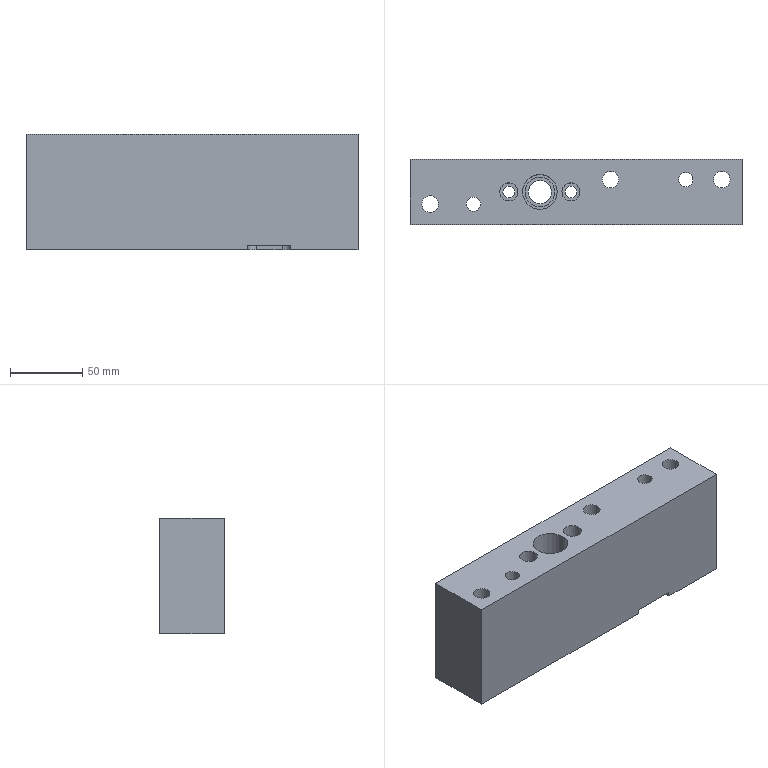Part | STEP file | lll_id2938_x_t | 1 solid | 44 faces | box 230 x 45 x 80 mm | volume 713661 mm3 | cylinder 23 | plane 19 | cone 2 | commonest cylinder face diameters 12 x4 12.5 x4 11.509 x3 18.007 x3 8.2 x2 8.505 x2
STEP:
#1=CARTESIAN_POINT('',(2997.75,0.,82.5));
#2=VERTEX_POINT('',#1);
#3=CARTESIAN_POINT('',(2991.5,0.,82.5));
#4=DIRECTION('',(0.,0.,-1.));
#5=DIRECTION('',(1.,0.,0.));
#6=AXIS2_PLACEMENT_3D('',#3,#4,#5);
#7=CIRCLE('',#6,6.25);
#8=EDGE_CURVE('',#2,#2,#7,.T.);
#9=ORIENTED_EDGE('',*,*,#8,.T.);
#10=EDGE_LOOP('',(#9));
#11=FACE_BOUND('',#10,.T.);
#12=CARTESIAN_POINT('',(2954.75,0.,82.5));
#13=VERTEX_POINT('',#12);
#14=CARTESIAN_POINT('',(2948.5,0.,82.5));
#15=DIRECTION('',(0.,0.,-1.));
#16=DIRECTION('',(1.,0.,0.));
#17=AXIS2_PLACEMENT_3D('',#14,#15,#16);
#18=CIRCLE('',#17,6.25);
#19=EDGE_CURVE('',#13,#13,#18,.T.);
#20=ORIENTED_EDGE('',*,*,#19,.T.);
#21=EDGE_LOOP('',(#20));
#22=FACE_BOUND('',#21,.T.);
#23=CARTESIAN_POINT('',(2919.,-8.5,82.5));
#24=VERTEX_POINT('',#23);
#25=CARTESIAN_POINT('',(2924.,-8.5,82.5));
#26=DIRECTION('',(0.,0.,1.));
#27=DIRECTION('',(-1.,0.,0.));
#28=AXIS2_PLACEMENT_3D('',#25,#26,#27);
#29=CIRCLE('',#28,5.);
#30=EDGE_CURVE('',#24,#24,#29,.T.);
#31=ORIENTED_EDGE('',*,*,#30,.F.);
#32=EDGE_LOOP('',(#31));
#33=FACE_BOUND('',#32,.T.);
#34=CARTESIAN_POINT('',(2888.245,-8.5,82.5));
#35=VERTEX_POINT('',#34);
#36=CARTESIAN_POINT('',(2894.,-8.5,82.5));
#37=DIRECTION('',(0.,0.,1.));
#38=DIRECTION('',(-1.,0.,0.));
#39=AXIS2_PLACEMENT_3D('',#36,#37,#38);
#40=CIRCLE('',#39,5.755);
#41=EDGE_CURVE('',#35,#35,#40,.T.);
#42=ORIENTED_EDGE('',*,*,#41,.F.);
#43=EDGE_LOOP('',(#42));
#44=FACE_BOUND('',#43,.T.);
#45=CARTESIAN_POINT('',(3013.245,8.5,82.5));
#46=VERTEX_POINT('',#45);
#47=CARTESIAN_POINT('',(3019.,8.5,82.5));
#48=DIRECTION('',(0.,0.,1.));
#49=DIRECTION('',(-1.,0.,0.));
#50=AXIS2_PLACEMENT_3D('',#47,#48,#49);
#51=CIRCLE('',#50,5.755);
#52=EDGE_CURVE('',#46,#46,#51,.T.);
#53=ORIENTED_EDGE('',*,*,#52,.F.);
#54=EDGE_LOOP('',(#53));
#55=FACE_BOUND('',#54,.T.);
#56=CARTESIAN_POINT('',(3090.245,8.5,82.5));
#57=VERTEX_POINT('',#56);
#58=CARTESIAN_POINT('',(3096.,8.5,82.5));
#59=DIRECTION('',(0.,0.,1.));
#60=DIRECTION('',(-1.,0.,0.));
#61=AXIS2_PLACEMENT_3D('',#58,#59,#60);
#62=CIRCLE('',#61,5.755);
#63=EDGE_CURVE('',#57,#57,#62,.T.);
#64=ORIENTED_EDGE('',*,*,#63,.F.);
#65=EDGE_LOOP('',(#64));
#66=FACE_BOUND('',#65,.T.);
#67=CARTESIAN_POINT('',(3066.,8.5,82.5));
#68=VERTEX_POINT('',#67);
#69=CARTESIAN_POINT('',(3071.,8.5,82.5));
#70=DIRECTION('',(0.,0.,1.));
#71=DIRECTION('',(-1.,0.,0.));
#72=AXIS2_PLACEMENT_3D('',#69,#70,#71);
#73=CIRCLE('',#72,5.);
#74=EDGE_CURVE('',#68,#68,#73,.T.);
#75=ORIENTED_EDGE('',*,*,#74,.F.);
#76=EDGE_LOOP('',(#75));
#77=FACE_BOUND('',#76,.T.);
#78=CARTESIAN_POINT('',(3110.,22.5,82.5));
#79=VERTEX_POINT('',#78);
#80=CARTESIAN_POINT('',(2880.,22.5,82.5));
#81=VERTEX_POINT('',#80);
#82=CARTESIAN_POINT('',(2940.,22.5,82.5));
#83=DIRECTION('',(-1.,0.,0.));
#84=VECTOR('',#83,1.);
#85=LINE('',#82,#84);
#86=EDGE_CURVE('',#79,#81,#85,.T.);
#87=ORIENTED_EDGE('',*,*,#86,.T.);
#88=CARTESIAN_POINT('',(2880.,-22.5,82.5));
#89=VERTEX_POINT('',#88);
#90=CARTESIAN_POINT('',(2880.,-216.1,82.5));
#91=DIRECTION('',(0.,1.,0.));
#92=VECTOR('',#91,1.);
#93=LINE('',#90,#92);
#94=EDGE_CURVE('',#89,#81,#93,.T.);
#95=ORIENTED_EDGE('',*,*,#94,.F.);
#96=CARTESIAN_POINT('',(3110.,-22.5,82.5));
#97=VERTEX_POINT('',#96);
#98=CARTESIAN_POINT('',(2715.34,-22.5,82.5));
#99=DIRECTION('',(1.,0.,0.));
#100=VECTOR('',#99,1.);
#101=LINE('',#98,#100);
#102=EDGE_CURVE('',#89,#97,#101,.T.);
#103=ORIENTED_EDGE('',*,*,#102,.T.);
#104=CARTESIAN_POINT('',(3110.,-216.1,82.5));
#105=DIRECTION('',(0.,1.,0.));
#106=VECTOR('',#105,1.);
#107=LINE('',#104,#106);
#108=EDGE_CURVE('',#97,#79,#107,.T.);
#109=ORIENTED_EDGE('',*,*,#108,.T.);
#110=EDGE_LOOP('',(#87,#95,#103,#109));
#111=FACE_BOUND('',#110,.T.);
#112=CARTESIAN_POINT('',(2982.,0.,82.5));
#113=VERTEX_POINT('',#112);
#114=CARTESIAN_POINT('',(2970.,0.,82.5));
#115=DIRECTION('',(0.,0.,-1.));
#116=DIRECTION('',(1.,0.,0.));
#117=AXIS2_PLACEMENT_3D('',#114,#115,#116);
#118=CIRCLE('',#117,12.);
#119=EDGE_CURVE('',#113,#113,#118,.T.);
#120=ORIENTED_EDGE('',*,*,#119,.T.);
#121=EDGE_LOOP('',(#120));
#122=FACE_BOUND('',#121,.T.);
#123=CARTESIAN_POINT('',(2940.,-216.1,82.5));
#124=DIRECTION('',(0.,0.,1.));
#125=DIRECTION('',(-1.,0.,0.));
#126=AXIS2_PLACEMENT_3D('',#123,#124,#125);
#127=PLANE('',#126);
#128=ADVANCED_FACE('',(#11,#22,#33,#44,#55,#66,#77,#111,#122),#127,.T.);
#129=CARTESIAN_POINT('',(2884.997,-8.5,2.5));
#130=VERTEX_POINT('',#129);
#131=CARTESIAN_POINT('',(2894.,-8.5,2.5));
#132=DIRECTION('',(0.,0.,1.));
#133=DIRECTION('',(-1.,0.,0.));
#134=AXIS2_PLACEMENT_3D('',#131,#132,#133);
#135=CIRCLE('',#134,9.004);
#136=EDGE_CURVE('',#130,#130,#135,.T.);
#137=ORIENTED_EDGE('',*,*,#136,.T.);
#138=EDGE_LOOP('',(#137));
#139=FACE_BOUND('',#138,.T.);
#140=CARTESIAN_POINT('',(2928.253,6.5,2.5));
#141=VERTEX_POINT('',#140);
#142=CARTESIAN_POINT('',(2924.,6.5,2.5));
#143=DIRECTION('',(0.,0.,1.));
#144=DIRECTION('',(1.,0.,0.));
#145=AXIS2_PLACEMENT_3D('',#142,#143,#144);
#146=CIRCLE('',#145,4.253);
#147=EDGE_CURVE('',#141,#141,#146,.T.);
#148=ORIENTED_EDGE('',*,*,#147,.T.);
#149=EDGE_LOOP('',(#148));
#150=FACE_BOUND('',#149,.T.);
#151=CARTESIAN_POINT('',(3110.,-22.5,2.5));
#152=VERTEX_POINT('',#151);
#153=CARTESIAN_POINT('',(3063.565,-22.5,2.5));
#154=VERTEX_POINT('',#153);
#155=CARTESIAN_POINT('',(2940.,-22.5,2.5));
#156=DIRECTION('',(-1.,0.,0.));
#157=VECTOR('',#156,1.);
#158=LINE('',#155,#157);
#159=EDGE_CURVE('',#152,#154,#158,.T.);
#160=ORIENTED_EDGE('',*,*,#159,.T.);
#161=CARTESIAN_POINT('',(3057.565,-16.5,2.5));
#162=VERTEX_POINT('',#161);
#163=CARTESIAN_POINT('',(3057.565,-22.5,2.5));
#164=DIRECTION('',(0.,0.,1.));
#165=DIRECTION('',(1.,0.,0.));
#166=AXIS2_PLACEMENT_3D('',#163,#164,#165);
#167=CIRCLE('',#166,6.);
#168=EDGE_CURVE('',#154,#162,#167,.T.);
#169=ORIENTED_EDGE('',*,*,#168,.T.);
#170=CARTESIAN_POINT('',(3039.565,-16.5,2.5));
#171=VERTEX_POINT('',#170);
#172=CARTESIAN_POINT('',(2940.,-16.5,2.5));
#173=DIRECTION('',(-1.,0.,0.));
#174=VECTOR('',#173,1.);
#175=LINE('',#172,#174);
#176=EDGE_CURVE('',#162,#171,#175,.T.);
#177=ORIENTED_EDGE('',*,*,#176,.T.);
#178=CARTESIAN_POINT('',(3033.565,-22.5,2.5));
#179=VERTEX_POINT('',#178);
#180=CARTESIAN_POINT('',(3039.565,-22.5,2.5));
#181=DIRECTION('',(0.,0.,1.));
#182=DIRECTION('',(1.,0.,0.));
#183=AXIS2_PLACEMENT_3D('',#180,#181,#182);
#184=CIRCLE('',#183,6.);
#185=EDGE_CURVE('',#171,#179,#184,.T.);
#186=ORIENTED_EDGE('',*,*,#185,.T.);
#187=CARTESIAN_POINT('',(2880.,-22.5,2.5));
#188=VERTEX_POINT('',#187);
#189=CARTESIAN_POINT('',(2940.,-22.5,2.5));
#190=DIRECTION('',(-1.,0.,0.));
#191=VECTOR('',#190,1.);
#192=LINE('',#189,#191);
#193=EDGE_CURVE('',#179,#188,#192,.T.);
#194=ORIENTED_EDGE('',*,*,#193,.T.);
#195=CARTESIAN_POINT('',(2880.,22.5,2.5));
#196=VERTEX_POINT('',#195);
#197=CARTESIAN_POINT('',(2880.,-26.737,2.5));
#198=DIRECTION('',(0.,1.,0.));
#199=VECTOR('',#198,1.);
#200=LINE('',#197,#199);
#201=EDGE_CURVE('',#188,#196,#200,.T.);
#202=ORIENTED_EDGE('',*,*,#201,.T.);
#203=CARTESIAN_POINT('',(3033.565,22.5,2.5));
#204=VERTEX_POINT('',#203);
#205=CARTESIAN_POINT('',(2940.,22.5,2.5));
#206=DIRECTION('',(1.,0.,0.));
#207=VECTOR('',#206,1.);
#208=LINE('',#205,#207);
#209=EDGE_CURVE('',#196,#204,#208,.T.);
#210=ORIENTED_EDGE('',*,*,#209,.T.);
#211=CARTESIAN_POINT('',(3039.565,16.5,2.5));
#212=VERTEX_POINT('',#211);
#213=CARTESIAN_POINT('',(3039.565,22.5,2.5));
#214=DIRECTION('',(0.,0.,1.));
#215=DIRECTION('',(1.,0.,0.));
#216=AXIS2_PLACEMENT_3D('',#213,#214,#215);
#217=CIRCLE('',#216,6.);
#218=EDGE_CURVE('',#204,#212,#217,.T.);
#219=ORIENTED_EDGE('',*,*,#218,.T.);
#220=CARTESIAN_POINT('',(3057.565,16.5,2.5));
#221=VERTEX_POINT('',#220);
#222=CARTESIAN_POINT('',(2940.,16.5,2.5));
#223=DIRECTION('',(1.,0.,0.));
#224=VECTOR('',#223,1.);
#225=LINE('',#222,#224);
#226=EDGE_CURVE('',#212,#221,#225,.T.);
#227=ORIENTED_EDGE('',*,*,#226,.T.);
#228=CARTESIAN_POINT('',(3063.565,22.5,2.5));
#229=VERTEX_POINT('',#228);
#230=CARTESIAN_POINT('',(3057.565,22.5,2.5));
#231=DIRECTION('',(0.,0.,1.));
#232=DIRECTION('',(1.,0.,0.));
#233=AXIS2_PLACEMENT_3D('',#230,#231,#232);
#234=CIRCLE('',#233,6.);
#235=EDGE_CURVE('',#221,#229,#234,.T.);
#236=ORIENTED_EDGE('',*,*,#235,.T.);
#237=CARTESIAN_POINT('',(3110.,22.5,2.5));
#238=VERTEX_POINT('',#237);
#239=CARTESIAN_POINT('',(2940.,22.5,2.5));
#240=DIRECTION('',(1.,0.,0.));
#241=VECTOR('',#240,1.);
#242=LINE('',#239,#241);
#243=EDGE_CURVE('',#229,#238,#242,.T.);
#244=ORIENTED_EDGE('',*,*,#243,.T.);
#245=CARTESIAN_POINT('',(3110.,-26.737,2.5));
#246=DIRECTION('',(0.,1.,0.));
#247=VECTOR('',#246,1.);
#248=LINE('',#245,#247);
#249=EDGE_CURVE('',#152,#238,#248,.T.);
#250=ORIENTED_EDGE('',*,*,#249,.F.);
#251=EDGE_LOOP('',(#160,#169,#177,#186,#194,#202,#210,#219,#227,#236,#244,#250));
#252=FACE_BOUND('',#251,.T.);
#253=CARTESIAN_POINT('',(2952.6,0.,2.5));
#254=VERTEX_POINT('',#253);
#255=CARTESIAN_POINT('',(2948.5,0.,2.5));
#256=DIRECTION('',(0.,0.,-1.));
#257=DIRECTION('',(1.,0.,0.));
#258=AXIS2_PLACEMENT_3D('',#255,#256,#257);
#259=CIRCLE('',#258,4.1);
#260=EDGE_CURVE('',#254,#254,#259,.T.);
#261=ORIENTED_EDGE('',*,*,#260,.F.);
#262=EDGE_LOOP('',(#261));
#263=FACE_BOUND('',#262,.T.);
#264=CARTESIAN_POINT('',(2995.6,0.,2.5));
#265=VERTEX_POINT('',#264);
#266=CARTESIAN_POINT('',(2991.5,0.,2.5));
#267=DIRECTION('',(0.,0.,-1.));
#268=DIRECTION('',(1.,0.,0.));
#269=AXIS2_PLACEMENT_3D('',#266,#267,#268);
#270=CIRCLE('',#269,4.1);
#271=EDGE_CURVE('',#265,#265,#270,.T.);
#272=ORIENTED_EDGE('',*,*,#271,.F.);
#273=EDGE_LOOP('',(#272));
#274=FACE_BOUND('',#273,.T.);
#275=CARTESIAN_POINT('',(3075.253,-6.5,2.5));
#276=VERTEX_POINT('',#275);
#277=CARTESIAN_POINT('',(3071.,-6.5,2.5));
#278=DIRECTION('',(0.,0.,1.));
#279=DIRECTION('',(1.,0.,0.));
#280=AXIS2_PLACEMENT_3D('',#277,#278,#279);
#281=CIRCLE('',#280,4.253);
#282=EDGE_CURVE('',#276,#276,#281,.T.);
#283=ORIENTED_EDGE('',*,*,#282,.T.);
#284=EDGE_LOOP('',(#283));
#285=FACE_BOUND('',#284,.T.);
#286=CARTESIAN_POINT('',(3064.75,8.5,2.5));
#287=VERTEX_POINT('',#286);
#288=CARTESIAN_POINT('',(3071.,8.5,2.5));
#289=DIRECTION('',(0.,0.,1.));
#290=DIRECTION('',(-1.,0.,0.));
#291=AXIS2_PLACEMENT_3D('',#288,#289,#290);
#292=CIRCLE('',#291,6.25);
#293=EDGE_CURVE('',#287,#287,#292,.T.);
#294=ORIENTED_EDGE('',*,*,#293,.T.);
#295=EDGE_LOOP('',(#294));
#296=FACE_BOUND('',#295,.T.);
#297=CARTESIAN_POINT('',(3086.997,8.5,2.5));
#298=VERTEX_POINT('',#297);
#299=CARTESIAN_POINT('',(3096.,8.5,2.5));
#300=DIRECTION('',(0.,0.,1.));
#301=DIRECTION('',(-1.,0.,0.));
#302=AXIS2_PLACEMENT_3D('',#299,#300,#301);
#303=CIRCLE('',#302,9.004);
#304=EDGE_CURVE('',#298,#298,#303,.T.);
#305=ORIENTED_EDGE('',*,*,#304,.T.);
#306=EDGE_LOOP('',(#305));
#307=FACE_BOUND('',#306,.T.);
#308=CARTESIAN_POINT('',(3009.997,8.5,2.5));
#309=VERTEX_POINT('',#308);
#310=CARTESIAN_POINT('',(3019.,8.5,2.5));
#311=DIRECTION('',(0.,0.,1.));
#312=DIRECTION('',(-1.,0.,0.));
#313=AXIS2_PLACEMENT_3D('',#310,#311,#312);
#314=CIRCLE('',#313,9.004);
#315=EDGE_CURVE('',#309,#309,#314,.T.);
#316=ORIENTED_EDGE('',*,*,#315,.T.);
#317=EDGE_LOOP('',(#316));
#318=FACE_BOUND('',#317,.T.);
#319=CARTESIAN_POINT('',(2917.75,-8.5,2.5));
#320=VERTEX_POINT('',#319);
#321=CARTESIAN_POINT('',(2924.,-8.5,2.5));
#322=DIRECTION('',(0.,0.,1.));
#323=DIRECTION('',(-1.,0.,0.));
#324=AXIS2_PLACEMENT_3D('',#321,#322,#323);
#325=CIRCLE('',#324,6.25);
#326=EDGE_CURVE('',#320,#320,#325,.T.);
#327=ORIENTED_EDGE('',*,*,#326,.T.);
#328=EDGE_LOOP('',(#327));
#329=FACE_BOUND('',#328,.T.);
#330=CARTESIAN_POINT('',(2978.,0.,2.5));
#331=VERTEX_POINT('',#330);
#332=CARTESIAN_POINT('',(2970.,0.,2.5));
#333=DIRECTION('',(0.,0.,1.));
#334=DIRECTION('',(1.,0.,0.));
#335=AXIS2_PLACEMENT_3D('',#332,#333,#334);
#336=CIRCLE('',#335,8.);
#337=EDGE_CURVE('',#331,#331,#336,.T.);
#338=ORIENTED_EDGE('',*,*,#337,.T.);
#339=EDGE_LOOP('',(#338));
#340=FACE_BOUND('',#339,.T.);
#341=CARTESIAN_POINT('',(2940.,-26.737,2.5));
#342=DIRECTION('',(0.,0.,1.));
#343=DIRECTION('',(-1.,0.,0.));
#344=AXIS2_PLACEMENT_3D('',#341,#342,#343);
#345=PLANE('',#344);
#346=ADVANCED_FACE('',(#139,#150,#252,#263,#274,#285,#296,#307,#318,#329,#340),#345,.F.);
#347=ORIENTED_EDGE('',*,*,#193,.F.);
#348=CARTESIAN_POINT('',(3033.565,-22.5,5.5));
#349=VERTEX_POINT('',#348);
#350=CARTESIAN_POINT('',(3033.565,-22.5,1307.5));
#351=DIRECTION('',(0.,0.,1.));
#352=VECTOR('',#351,1.);
#353=LINE('',#350,#352);
#354=EDGE_CURVE('',#179,#349,#353,.T.);
#355=ORIENTED_EDGE('',*,*,#354,.T.);
#356=CARTESIAN_POINT('',(3063.565,-22.5,5.5));
#357=VERTEX_POINT('',#356);
#358=CARTESIAN_POINT('',(2715.34,-22.5,5.5));
#359=DIRECTION('',(1.,0.,0.));
#360=VECTOR('',#359,1.);
#361=LINE('',#358,#360);
#362=EDGE_CURVE('',#349,#357,#361,.T.);
#363=ORIENTED_EDGE('',*,*,#362,.T.);
#364=CARTESIAN_POINT('',(3063.565,-22.5,1307.5));
#365=DIRECTION('',(0.,0.,-1.));
#366=VECTOR('',#365,1.);
#367=LINE('',#364,#366);
#368=EDGE_CURVE('',#357,#154,#367,.T.);
#369=ORIENTED_EDGE('',*,*,#368,.T.);
#370=ORIENTED_EDGE('',*,*,#159,.F.);
#371=CARTESIAN_POINT('',(3110.,-22.5,12.5));
#372=DIRECTION('',(0.,0.,1.));
#373=VECTOR('',#372,1.);
#374=LINE('',#371,#373);
#375=EDGE_CURVE('',#152,#97,#374,.T.);
#376=ORIENTED_EDGE('',*,*,#375,.T.);
#377=ORIENTED_EDGE('',*,*,#102,.F.);
#378=CARTESIAN_POINT('',(2880.,-22.5,1307.5));
#379=DIRECTION('',(0.,0.,-1.));
#380=VECTOR('',#379,1.);
#381=LINE('',#378,#380);
#382=EDGE_CURVE('',#89,#188,#381,.T.);
#383=ORIENTED_EDGE('',*,*,#382,.T.);
#384=EDGE_LOOP('',(#347,#355,#363,#369,#370,#376,#377,#383));
#385=FACE_OUTER_BOUND('',#384,.T.);
#386=CARTESIAN_POINT('',(2715.34,-22.5,1307.5));
#387=DIRECTION('',(0.,1.,0.));
#388=DIRECTION('',(0.,0.,-1.));
#389=AXIS2_PLACEMENT_3D('',#386,#387,#388);
#390=PLANE('',#389);
#391=ADVANCED_FACE('',(#385),#390,.F.);
#392=CARTESIAN_POINT('',(3110.,22.5,52.5));
#393=DIRECTION('',(0.,0.,1.));
#394=VECTOR('',#393,1.);
#395=LINE('',#392,#394);
#396=EDGE_CURVE('',#238,#79,#395,.T.);
#397=ORIENTED_EDGE('',*,*,#396,.T.);
#398=ORIENTED_EDGE('',*,*,#108,.F.);
#399=ORIENTED_EDGE('',*,*,#375,.F.);
#400=ORIENTED_EDGE('',*,*,#249,.T.);
#401=EDGE_LOOP('',(#397,#398,#399,#400));
#402=FACE_OUTER_BOUND('',#401,.T.);
#403=CARTESIAN_POINT('',(3110.,26.737,12.5));
#404=DIRECTION('',(1.,0.,0.));
#405=DIRECTION('',(0.,0.,1.));
#406=AXIS2_PLACEMENT_3D('',#403,#404,#405);
#407=PLANE('',#406);
#408=ADVANCED_FACE('',(#402),#407,.T.);
#409=ORIENTED_EDGE('',*,*,#94,.T.);
#410=CARTESIAN_POINT('',(2880.,22.5,12.5));
#411=DIRECTION('',(0.,0.,-1.));
#412=VECTOR('',#411,1.);
#413=LINE('',#410,#412);
#414=EDGE_CURVE('',#81,#196,#413,.T.);
#415=ORIENTED_EDGE('',*,*,#414,.T.);
#416=ORIENTED_EDGE('',*,*,#201,.F.);
#417=ORIENTED_EDGE('',*,*,#382,.F.);
#418=EDGE_LOOP('',(#409,#415,#416,#417));
#419=FACE_OUTER_BOUND('',#418,.T.);
#420=CARTESIAN_POINT('',(2880.,26.737,12.5));
#421=DIRECTION('',(1.,0.,0.));
#422=DIRECTION('',(0.,0.,1.));
#423=AXIS2_PLACEMENT_3D('',#420,#421,#422);
#424=PLANE('',#423);
#425=ADVANCED_FACE('',(#419),#424,.F.);
#426=CARTESIAN_POINT('',(3063.565,22.5,5.5));
#427=VERTEX_POINT('',#426);
#428=CARTESIAN_POINT('',(3033.565,22.5,5.5));
#429=VERTEX_POINT('',#428);
#430=CARTESIAN_POINT('',(2940.,22.5,5.5));
#431=DIRECTION('',(-1.,0.,0.));
#432=VECTOR('',#431,1.);
#433=LINE('',#430,#432);
#434=EDGE_CURVE('',#427,#429,#433,.T.);
#435=ORIENTED_EDGE('',*,*,#434,.T.);
#436=CARTESIAN_POINT('',(3033.565,22.5,52.5));
#437=DIRECTION('',(0.,0.,-1.));
#438=VECTOR('',#437,1.);
#439=LINE('',#436,#438);
#440=EDGE_CURVE('',#429,#204,#439,.T.);
#441=ORIENTED_EDGE('',*,*,#440,.T.);
#442=ORIENTED_EDGE('',*,*,#209,.F.);
#443=ORIENTED_EDGE('',*,*,#414,.F.);
#444=ORIENTED_EDGE('',*,*,#86,.F.);
#445=ORIENTED_EDGE('',*,*,#396,.F.);
#446=ORIENTED_EDGE('',*,*,#243,.F.);
#447=CARTESIAN_POINT('',(3063.565,22.5,52.5));
#448=DIRECTION('',(0.,0.,1.));
#449=VECTOR('',#448,1.);
#450=LINE('',#447,#449);
#451=EDGE_CURVE('',#229,#427,#450,.T.);
#452=ORIENTED_EDGE('',*,*,#451,.T.);
#453=EDGE_LOOP('',(#435,#441,#442,#443,#444,#445,#446,#452));
#454=FACE_OUTER_BOUND('',#453,.T.);
#455=CARTESIAN_POINT('',(2940.,22.5,52.5));
#456=DIRECTION('',(0.,-1.,0.));
#457=DIRECTION('',(0.,0.,1.));
#458=AXIS2_PLACEMENT_3D('',#455,#456,#457);
#459=PLANE('',#458);
#460=ADVANCED_FACE('',(#454),#459,.F.);
#461=CARTESIAN_POINT('',(3064.75,8.5,43.5));
#462=VERTEX_POINT('',#461);
#463=CARTESIAN_POINT('',(3071.,8.5,43.5));
#464=DIRECTION('',(0.,0.,1.));
#465=DIRECTION('',(-1.,0.,0.));
#466=AXIS2_PLACEMENT_3D('',#463,#464,#465);
#467=CIRCLE('',#466,6.25);
#468=EDGE_CURVE('',#462,#462,#467,.T.);
#469=ORIENTED_EDGE('',*,*,#468,.T.);
#470=EDGE_LOOP('',(#469));
#471=FACE_BOUND('',#470,.T.);
#472=ORIENTED_EDGE('',*,*,#293,.F.);
#473=EDGE_LOOP('',(#472));
#474=FACE_BOUND('',#473,.T.);
#475=CARTESIAN_POINT('',(3071.,8.5,-2.5));
#476=DIRECTION('',(0.,0.,1.));
#477=DIRECTION('',(-1.,0.,0.));
#478=AXIS2_PLACEMENT_3D('',#475,#476,#477);
#479=CYLINDRICAL_SURFACE('',#478,6.25);
#480=ADVANCED_FACE('',(#471,#474),#479,.F.);
#481=ORIENTED_EDGE('',*,*,#74,.T.);
#482=EDGE_LOOP('',(#481));
#483=FACE_BOUND('',#482,.T.);
#484=CARTESIAN_POINT('',(3066.,8.5,43.5));
#485=VERTEX_POINT('',#484);
#486=CARTESIAN_POINT('',(3071.,8.5,43.5));
#487=DIRECTION('',(0.,0.,1.));
#488=DIRECTION('',(-1.,0.,0.));
#489=AXIS2_PLACEMENT_3D('',#486,#487,#488);
#490=CIRCLE('',#489,5.);
#491=EDGE_CURVE('',#485,#485,#490,.T.);
#492=ORIENTED_EDGE('',*,*,#491,.F.);
#493=EDGE_LOOP('',(#492));
#494=FACE_BOUND('',#493,.T.);
#495=CARTESIAN_POINT('',(3071.,8.5,-2.5));
#496=DIRECTION('',(0.,0.,1.));
#497=DIRECTION('',(-1.,0.,0.));
#498=AXIS2_PLACEMENT_3D('',#495,#496,#497);
#499=CYLINDRICAL_SURFACE('',#498,5.);
#500=ADVANCED_FACE('',(#483,#494),#499,.F.);
#501=ORIENTED_EDGE('',*,*,#491,.T.);
#502=EDGE_LOOP('',(#501));
#503=FACE_BOUND('',#502,.T.);
#504=ORIENTED_EDGE('',*,*,#468,.F.);
#505=EDGE_LOOP('',(#504));
#506=FACE_BOUND('',#505,.T.);
#507=CARTESIAN_POINT('',(3071.,8.5,43.5));
#508=DIRECTION('',(0.,0.,1.));
#509=DIRECTION('',(-1.,0.,0.));
#510=AXIS2_PLACEMENT_3D('',#507,#508,#509);
#511=PLANE('',#510);
#512=ADVANCED_FACE('',(#503,#506),#511,.F.);
#513=ORIENTED_EDGE('',*,*,#63,.T.);
#514=EDGE_LOOP('',(#513));
#515=FACE_BOUND('',#514,.T.);
#516=CARTESIAN_POINT('',(3090.245,8.5,52.5));
#517=VERTEX_POINT('',#516);
#518=CARTESIAN_POINT('',(3096.,8.5,52.5));
#519=DIRECTION('',(0.,0.,1.));
#520=DIRECTION('',(-1.,0.,0.));
#521=AXIS2_PLACEMENT_3D('',#518,#519,#520);
#522=CIRCLE('',#521,5.755);
#523=EDGE_CURVE('',#517,#517,#522,.T.);
#524=ORIENTED_EDGE('',*,*,#523,.F.);
#525=EDGE_LOOP('',(#524));
#526=FACE_BOUND('',#525,.T.);
#527=CARTESIAN_POINT('',(3096.,8.5,-2.5));
#528=DIRECTION('',(0.,0.,1.));
#529=DIRECTION('',(-1.,0.,0.));
#530=AXIS2_PLACEMENT_3D('',#527,#528,#529);
#531=CYLINDRICAL_SURFACE('',#530,5.755);
#532=ADVANCED_FACE('',(#515,#526),#531,.F.);
#533=ORIENTED_EDGE('',*,*,#523,.T.);
#534=EDGE_LOOP('',(#533));
#535=FACE_BOUND('',#534,.T.);
#536=CARTESIAN_POINT('',(3086.997,8.5,52.5));
#537=VERTEX_POINT('',#536);
#538=CARTESIAN_POINT('',(3096.,8.5,52.5));
#539=DIRECTION('',(0.,0.,1.));
#540=DIRECTION('',(-1.,0.,0.));
#541=AXIS2_PLACEMENT_3D('',#538,#539,#540);
#542=CIRCLE('',#541,9.004);
#543=EDGE_CURVE('',#537,#537,#542,.T.);
#544=ORIENTED_EDGE('',*,*,#543,.F.);
#545=EDGE_LOOP('',(#544));
#546=FACE_BOUND('',#545,.T.);
#547=CARTESIAN_POINT('',(3096.,8.5,52.5));
#548=DIRECTION('',(0.,0.,1.));
#549=DIRECTION('',(-1.,0.,0.));
#550=AXIS2_PLACEMENT_3D('',#547,#548,#549);
#551=PLANE('',#550);
#552=ADVANCED_FACE('',(#535,#546),#551,.F.);
#553=ORIENTED_EDGE('',*,*,#543,.T.);
#554=EDGE_LOOP('',(#553));
#555=FACE_BOUND('',#554,.T.);
#556=ORIENTED_EDGE('',*,*,#304,.F.);
#557=EDGE_LOOP('',(#556));
#558=FACE_BOUND('',#557,.T.);
#559=CARTESIAN_POINT('',(3096.,8.5,2.5));
#560=DIRECTION('',(0.,0.,1.));
#561=DIRECTION('',(-1.,0.,0.));
#562=AXIS2_PLACEMENT_3D('',#559,#560,#561);
#563=CYLINDRICAL_SURFACE('',#562,9.004);
#564=ADVANCED_FACE('',(#555,#558),#563,.F.);
#565=ORIENTED_EDGE('',*,*,#52,.T.);
#566=EDGE_LOOP('',(#565));
#567=FACE_BOUND('',#566,.T.);
#568=CARTESIAN_POINT('',(3013.245,8.5,52.5));
#569=VERTEX_POINT('',#568);
#570=CARTESIAN_POINT('',(3019.,8.5,52.5));
#571=DIRECTION('',(0.,0.,1.));
#572=DIRECTION('',(-1.,0.,0.));
#573=AXIS2_PLACEMENT_3D('',#570,#571,#572);
#574=CIRCLE('',#573,5.755);
#575=EDGE_CURVE('',#569,#569,#574,.T.);
#576=ORIENTED_EDGE('',*,*,#575,.F.);
#577=EDGE_LOOP('',(#576));
#578=FACE_BOUND('',#577,.T.);
#579=CARTESIAN_POINT('',(3019.,8.5,-2.5));
#580=DIRECTION('',(0.,0.,1.));
#581=DIRECTION('',(-1.,0.,0.));
#582=AXIS2_PLACEMENT_3D('',#579,#580,#581);
#583=CYLINDRICAL_SURFACE('',#582,5.755);
#584=ADVANCED_FACE('',(#567,#578),#583,.F.);
#585=ORIENTED_EDGE('',*,*,#575,.T.);
#586=EDGE_LOOP('',(#585));
#587=FACE_BOUND('',#586,.T.);
#588=CARTESIAN_POINT('',(3009.997,8.5,52.5));
#589=VERTEX_POINT('',#588);
#590=CARTESIAN_POINT('',(3019.,8.5,52.5));
#591=DIRECTION('',(0.,0.,1.));
#592=DIRECTION('',(-1.,0.,0.));
#593=AXIS2_PLACEMENT_3D('',#590,#591,#592);
#594=CIRCLE('',#593,9.004);
#595=EDGE_CURVE('',#589,#589,#594,.T.);
#596=ORIENTED_EDGE('',*,*,#595,.F.);
#597=EDGE_LOOP('',(#596));
#598=FACE_BOUND('',#597,.T.);
#599=CARTESIAN_POINT('',(3019.,8.5,52.5));
#600=DIRECTION('',(0.,0.,1.));
#601=DIRECTION('',(-1.,0.,0.));
#602=AXIS2_PLACEMENT_3D('',#599,#600,#601);
#603=PLANE('',#602);
#604=ADVANCED_FACE('',(#587,#598),#603,.F.);
#605=ORIENTED_EDGE('',*,*,#595,.T.);
#606=EDGE_LOOP('',(#605));
#607=FACE_BOUND('',#606,.T.);
#608=ORIENTED_EDGE('',*,*,#315,.F.);
#609=EDGE_LOOP('',(#608));
#610=FACE_BOUND('',#609,.T.);
#611=CARTESIAN_POINT('',(3019.,8.5,2.5));
#612=DIRECTION('',(0.,0.,1.));
#613=DIRECTION('',(-1.,0.,0.));
#614=AXIS2_PLACEMENT_3D('',#611,#612,#613);
#615=CYLINDRICAL_SURFACE('',#614,9.004);
#616=ADVANCED_FACE('',(#607,#610),#615,.F.);
#617=ORIENTED_EDGE('',*,*,#41,.T.);
#618=EDGE_LOOP('',(#617));
#619=FACE_BOUND('',#618,.T.);
#620=CARTESIAN_POINT('',(2888.245,-8.5,52.5));
#621=VERTEX_POINT('',#620);
#622=CARTESIAN_POINT('',(2894.,-8.5,52.5));
#623=DIRECTION('',(0.,0.,1.));
#624=DIRECTION('',(-1.,0.,0.));
#625=AXIS2_PLACEMENT_3D('',#622,#623,#624);
#626=CIRCLE('',#625,5.755);
#627=EDGE_CURVE('',#621,#621,#626,.T.);
#628=ORIENTED_EDGE('',*,*,#627,.F.);
#629=EDGE_LOOP('',(#628));
#630=FACE_BOUND('',#629,.T.);
#631=CARTESIAN_POINT('',(2894.,-8.5,-2.5));
#632=DIRECTION('',(0.,0.,1.));
#633=DIRECTION('',(-1.,0.,0.));
#634=AXIS2_PLACEMENT_3D('',#631,#632,#633);
#635=CYLINDRICAL_SURFACE('',#634,5.755);
#636=ADVANCED_FACE('',(#619,#630),#635,.F.);
#637=ORIENTED_EDGE('',*,*,#627,.T.);
#638=EDGE_LOOP('',(#637));
#639=FACE_BOUND('',#638,.T.);
#640=CARTESIAN_POINT('',(2884.997,-8.5,52.5));
#641=VERTEX_POINT('',#640);
#642=CARTESIAN_POINT('',(2894.,-8.5,52.5));
#643=DIRECTION('',(0.,0.,1.));
#644=DIRECTION('',(-1.,0.,0.));
#645=AXIS2_PLACEMENT_3D('',#642,#643,#644);
#646=CIRCLE('',#645,9.004);
#647=EDGE_CURVE('',#641,#641,#646,.T.);
#648=ORIENTED_EDGE('',*,*,#647,.F.);
#649=EDGE_LOOP('',(#648));
#650=FACE_BOUND('',#649,.T.);
#651=CARTESIAN_POINT('',(2894.,-8.5,52.5));
#652=DIRECTION('',(0.,0.,1.));
#653=DIRECTION('',(-1.,0.,0.));
#654=AXIS2_PLACEMENT_3D('',#651,#652,#653);
#655=PLANE('',#654);
#656=ADVANCED_FACE('',(#639,#650),#655,.F.);
#657=ORIENTED_EDGE('',*,*,#647,.T.);
#658=EDGE_LOOP('',(#657));
#659=FACE_BOUND('',#658,.T.);
#660=ORIENTED_EDGE('',*,*,#136,.F.);
#661=EDGE_LOOP('',(#660));
#662=FACE_BOUND('',#661,.T.);
#663=CARTESIAN_POINT('',(2894.,-8.5,2.5));
#664=DIRECTION('',(0.,0.,1.));
#665=DIRECTION('',(-1.,0.,0.));
#666=AXIS2_PLACEMENT_3D('',#663,#664,#665);
#667=CYLINDRICAL_SURFACE('',#666,9.004);
#668=ADVANCED_FACE('',(#659,#662),#667,.F.);
#669=CARTESIAN_POINT('',(2917.75,-8.5,43.5));
#670=VERTEX_POINT('',#669);
#671=CARTESIAN_POINT('',(2924.,-8.5,43.5));
#672=DIRECTION('',(0.,0.,1.));
#673=DIRECTION('',(-1.,0.,0.));
#674=AXIS2_PLACEMENT_3D('',#671,#672,#673);
#675=CIRCLE('',#674,6.25);
#676=EDGE_CURVE('',#670,#670,#675,.T.);
#677=ORIENTED_EDGE('',*,*,#676,.T.);
#678=EDGE_LOOP('',(#677));
#679=FACE_BOUND('',#678,.T.);
#680=ORIENTED_EDGE('',*,*,#326,.F.);
#681=EDGE_LOOP('',(#680));
#682=FACE_BOUND('',#681,.T.);
#683=CARTESIAN_POINT('',(2924.,-8.5,-2.5));
#684=DIRECTION('',(0.,0.,1.));
#685=DIRECTION('',(-1.,0.,0.));
#686=AXIS2_PLACEMENT_3D('',#683,#684,#685);
#687=CYLINDRICAL_SURFACE('',#686,6.25);
#688=ADVANCED_FACE('',(#679,#682),#687,.F.);
#689=ORIENTED_EDGE('',*,*,#30,.T.);
#690=EDGE_LOOP('',(#689));
#691=FACE_BOUND('',#690,.T.);
#692=CARTESIAN_POINT('',(2919.,-8.5,43.5));
#693=VERTEX_POINT('',#692);
#694=CARTESIAN_POINT('',(2924.,-8.5,43.5));
#695=DIRECTION('',(0.,0.,1.));
#696=DIRECTION('',(-1.,0.,0.));
#697=AXIS2_PLACEMENT_3D('',#694,#695,#696);
#698=CIRCLE('',#697,5.);
#699=EDGE_CURVE('',#693,#693,#698,.T.);
#700=ORIENTED_EDGE('',*,*,#699,.F.);
#701=EDGE_LOOP('',(#700));
#702=FACE_BOUND('',#701,.T.);
#703=CARTESIAN_POINT('',(2924.,-8.5,-2.5));
#704=DIRECTION('',(0.,0.,1.));
#705=DIRECTION('',(-1.,0.,0.));
#706=AXIS2_PLACEMENT_3D('',#703,#704,#705);
#707=CYLINDRICAL_SURFACE('',#706,5.);
#708=ADVANCED_FACE('',(#691,#702),#707,.F.);
#709=ORIENTED_EDGE('',*,*,#699,.T.);
#710=EDGE_LOOP('',(#709));
#711=FACE_BOUND('',#710,.T.);
#712=ORIENTED_EDGE('',*,*,#676,.F.);
#713=EDGE_LOOP('',(#712));
#714=FACE_BOUND('',#713,.T.);
#715=CARTESIAN_POINT('',(2924.,-8.5,43.5));
#716=DIRECTION('',(0.,0.,1.));
#717=DIRECTION('',(-1.,0.,0.));
#718=AXIS2_PLACEMENT_3D('',#715,#716,#717);
#719=PLANE('',#718);
#720=ADVANCED_FACE('',(#711,#714),#719,.F.);
#721=CARTESIAN_POINT('',(3075.253,-6.5,33.254));
#722=VERTEX_POINT('',#721);
#723=CARTESIAN_POINT('',(3071.,-6.5,33.254));
#724=DIRECTION('',(0.,0.,1.));
#725=DIRECTION('',(1.,0.,0.));
#726=AXIS2_PLACEMENT_3D('',#723,#724,#725);
#727=CIRCLE('',#726,4.253);
#728=EDGE_CURVE('',#722,#722,#727,.T.);
#729=ORIENTED_EDGE('',*,*,#728,.T.);
#730=EDGE_LOOP('',(#729));
#731=FACE_BOUND('',#730,.T.);
#732=ORIENTED_EDGE('',*,*,#282,.F.);
#733=EDGE_LOOP('',(#732));
#734=FACE_BOUND('',#733,.T.);
#735=CARTESIAN_POINT('',(3071.,-6.5,2.5));
#736=DIRECTION('',(0.,0.,1.));
#737=DIRECTION('',(1.,0.,0.));
#738=AXIS2_PLACEMENT_3D('',#735,#736,#737);
#739=CYLINDRICAL_SURFACE('',#738,4.253);
#740=ADVANCED_FACE('',(#731,#734),#739,.F.);
#741=CARTESIAN_POINT('',(3071.,-6.5,37.506));
#742=VERTEX_POINT('',#741);
#743=VERTEX_LOOP('',#742);
#744=FACE_BOUND('',#743,.T.);
#745=ORIENTED_EDGE('',*,*,#728,.F.);
#746=EDGE_LOOP('',(#745));
#747=FACE_BOUND('',#746,.T.);
#748=CARTESIAN_POINT('',(3071.,-6.5,33.254));
#749=DIRECTION('',(0.,0.,-1.));
#750=DIRECTION('',(-1.,0.,0.));
#751=AXIS2_PLACEMENT_3D('',#748,#749,#750);
#752=CONICAL_SURFACE('',#751,4.253,45.);
#753=ADVANCED_FACE('',(#744,#747),#752,.F.);
#754=CARTESIAN_POINT('',(2928.253,6.5,33.254));
#755=VERTEX_POINT('',#754);
#756=CARTESIAN_POINT('',(2924.,6.5,33.254));
#757=DIRECTION('',(0.,0.,1.));
#758=DIRECTION('',(1.,0.,0.));
#759=AXIS2_PLACEMENT_3D('',#756,#757,#758);
#760=CIRCLE('',#759,4.253);
#761=EDGE_CURVE('',#755,#755,#760,.T.);
#762=ORIENTED_EDGE('',*,*,#761,.T.);
#763=EDGE_LOOP('',(#762));
#764=FACE_BOUND('',#763,.T.);
#765=ORIENTED_EDGE('',*,*,#147,.F.);
#766=EDGE_LOOP('',(#765));
#767=FACE_BOUND('',#766,.T.);
#768=CARTESIAN_POINT('',(2924.,6.5,2.5));
#769=DIRECTION('',(0.,0.,1.));
#770=DIRECTION('',(1.,0.,0.));
#771=AXIS2_PLACEMENT_3D('',#768,#769,#770);
#772=CYLINDRICAL_SURFACE('',#771,4.253);
#773=ADVANCED_FACE('',(#764,#767),#772,.F.);
#774=CARTESIAN_POINT('',(2924.,6.5,37.506));
#775=VERTEX_POINT('',#774);
#776=VERTEX_LOOP('',#775);
#777=FACE_BOUND('',#776,.T.);
#778=ORIENTED_EDGE('',*,*,#761,.F.);
#779=EDGE_LOOP('',(#778));
#780=FACE_BOUND('',#779,.T.);
#781=CARTESIAN_POINT('',(2924.,6.5,33.254));
#782=DIRECTION('',(0.,0.,-1.));
#783=DIRECTION('',(-1.,0.,0.));
#784=AXIS2_PLACEMENT_3D('',#781,#782,#783);
#785=CONICAL_SURFACE('',#784,4.253,45.);
#786=ADVANCED_FACE('',(#777,#780),#785,.F.);
#787=CARTESIAN_POINT('',(2944.4,0.,22.5));
#788=VERTEX_POINT('',#787);
#789=CARTESIAN_POINT('',(2948.5,0.,22.5));
#790=DIRECTION('',(0.,0.,1.));
#791=DIRECTION('',(-1.,0.,0.));
#792=AXIS2_PLACEMENT_3D('',#789,#790,#791);
#793=CIRCLE('',#792,4.1);
#794=EDGE_CURVE('',#788,#788,#793,.T.);
#795=ORIENTED_EDGE('',*,*,#794,.T.);
#796=EDGE_LOOP('',(#795));
#797=FACE_BOUND('',#796,.T.);
#798=ORIENTED_EDGE('',*,*,#260,.T.);
#799=EDGE_LOOP('',(#798));
#800=FACE_BOUND('',#799,.T.);
#801=CARTESIAN_POINT('',(2948.5,0.,-2.5));
#802=DIRECTION('',(0.,0.,1.));
#803=DIRECTION('',(1.,0.,0.));
#804=AXIS2_PLACEMENT_3D('',#801,#802,#803);
#805=CYLINDRICAL_SURFACE('',#804,4.1);
#806=ADVANCED_FACE('',(#797,#800),#805,.F.);
#807=CARTESIAN_POINT('',(2942.25,0.,22.5));
#808=VERTEX_POINT('',#807);
#809=CARTESIAN_POINT('',(2948.5,0.,22.5));
#810=DIRECTION('',(0.,0.,-1.));
#811=DIRECTION('',(-1.,0.,0.));
#812=AXIS2_PLACEMENT_3D('',#809,#810,#811);
#813=CIRCLE('',#812,6.25);
#814=EDGE_CURVE('',#808,#808,#813,.T.);
#815=ORIENTED_EDGE('',*,*,#814,.F.);
#816=EDGE_LOOP('',(#815));
#817=FACE_BOUND('',#816,.T.);
#818=ORIENTED_EDGE('',*,*,#794,.F.);
#819=EDGE_LOOP('',(#818));
#820=FACE_BOUND('',#819,.T.);
#821=CARTESIAN_POINT('',(2948.5,0.,22.5));
#822=DIRECTION('',(0.,0.,-1.));
#823=DIRECTION('',(-1.,0.,0.));
#824=AXIS2_PLACEMENT_3D('',#821,#822,#823);
#825=PLANE('',#824);
#826=ADVANCED_FACE('',(#817,#820),#825,.F.);
#827=ORIENTED_EDGE('',*,*,#19,.F.);
#828=EDGE_LOOP('',(#827));
#829=FACE_BOUND('',#828,.T.);
#830=ORIENTED_EDGE('',*,*,#814,.T.);
#831=EDGE_LOOP('',(#830));
#832=FACE_BOUND('',#831,.T.);
#833=CARTESIAN_POINT('',(2948.5,0.,27.5));
#834=DIRECTION('',(0.,0.,1.));
#835=DIRECTION('',(1.,0.,0.));
#836=AXIS2_PLACEMENT_3D('',#833,#834,#835);
#837=CYLINDRICAL_SURFACE('',#836,6.25);
#838=ADVANCED_FACE('',(#829,#832),#837,.F.);
#839=CARTESIAN_POINT('',(2987.4,0.,22.5));
#840=VERTEX_POINT('',#839);
#841=CARTESIAN_POINT('',(2991.5,0.,22.5));
#842=DIRECTION('',(0.,0.,1.));
#843=DIRECTION('',(-1.,0.,0.));
#844=AXIS2_PLACEMENT_3D('',#841,#842,#843);
#845=CIRCLE('',#844,4.1);
#846=EDGE_CURVE('',#840,#840,#845,.T.);
#847=ORIENTED_EDGE('',*,*,#846,.T.);
#848=EDGE_LOOP('',(#847));
#849=FACE_BOUND('',#848,.T.);
#850=ORIENTED_EDGE('',*,*,#271,.T.);
#851=EDGE_LOOP('',(#850));
#852=FACE_BOUND('',#851,.T.);
#853=CARTESIAN_POINT('',(2991.5,0.,-2.));
#854=DIRECTION('',(0.,0.,1.));
#855=DIRECTION('',(1.,0.,0.));
#856=AXIS2_PLACEMENT_3D('',#853,#854,#855);
#857=CYLINDRICAL_SURFACE('',#856,4.1);
#858=ADVANCED_FACE('',(#849,#852),#857,.F.);
#859=CARTESIAN_POINT('',(2985.25,0.,22.5));
#860=VERTEX_POINT('',#859);
#861=CARTESIAN_POINT('',(2991.5,0.,22.5));
#862=DIRECTION('',(0.,0.,-1.));
#863=DIRECTION('',(-1.,0.,0.));
#864=AXIS2_PLACEMENT_3D('',#861,#862,#863);
#865=CIRCLE('',#864,6.25);
#866=EDGE_CURVE('',#860,#860,#865,.T.);
#867=ORIENTED_EDGE('',*,*,#866,.F.);
#868=EDGE_LOOP('',(#867));
#869=FACE_BOUND('',#868,.T.);
#870=ORIENTED_EDGE('',*,*,#846,.F.);
#871=EDGE_LOOP('',(#870));
#872=FACE_BOUND('',#871,.T.);
#873=CARTESIAN_POINT('',(2991.5,0.,22.5));
#874=DIRECTION('',(0.,0.,-1.));
#875=DIRECTION('',(-1.,0.,0.));
#876=AXIS2_PLACEMENT_3D('',#873,#874,#875);
#877=PLANE('',#876);
#878=ADVANCED_FACE('',(#869,#872),#877,.F.);
#879=ORIENTED_EDGE('',*,*,#8,.F.);
#880=EDGE_LOOP('',(#879));
#881=FACE_BOUND('',#880,.T.);
#882=ORIENTED_EDGE('',*,*,#866,.T.);
#883=EDGE_LOOP('',(#882));
#884=FACE_BOUND('',#883,.T.);
#885=CARTESIAN_POINT('',(2991.5,0.,27.5));
#886=DIRECTION('',(0.,0.,1.));
#887=DIRECTION('',(1.,0.,0.));
#888=AXIS2_PLACEMENT_3D('',#885,#886,#887);
#889=CYLINDRICAL_SURFACE('',#888,6.25);
#890=ADVANCED_FACE('',(#881,#884),#889,.F.);
#891=CARTESIAN_POINT('',(2959.75,0.,42.5));
#892=VERTEX_POINT('',#891);
#893=CARTESIAN_POINT('',(2970.,0.,42.5));
#894=DIRECTION('',(0.,0.,-1.));
#895=DIRECTION('',(-1.,0.,0.));
#896=AXIS2_PLACEMENT_3D('',#893,#894,#895);
#897=CIRCLE('',#896,10.25);
#898=EDGE_CURVE('',#892,#892,#897,.T.);
#899=ORIENTED_EDGE('',*,*,#898,.F.);
#900=EDGE_LOOP('',(#899));
#901=FACE_BOUND('',#900,.T.);
#902=CARTESIAN_POINT('',(2959.75,0.,19.5));
#903=VERTEX_POINT('',#902);
#904=CARTESIAN_POINT('',(2970.,0.,19.5));
#905=DIRECTION('',(0.,0.,1.));
#906=DIRECTION('',(-1.,0.,0.));
#907=AXIS2_PLACEMENT_3D('',#904,#905,#906);
#908=CIRCLE('',#907,10.25);
#909=EDGE_CURVE('',#903,#903,#908,.T.);
#910=ORIENTED_EDGE('',*,*,#909,.F.);
#911=EDGE_LOOP('',(#910));
#912=FACE_BOUND('',#911,.T.);
#913=CARTESIAN_POINT('',(2970.,0.,24.5));
#914=DIRECTION('',(0.,0.,-1.));
#915=DIRECTION('',(0.,1.,0.));
#916=AXIS2_PLACEMENT_3D('',#913,#914,#915);
#917=CYLINDRICAL_SURFACE('',#916,10.25);
#918=ADVANCED_FACE('',(#901,#912),#917,.F.);
#919=CARTESIAN_POINT('',(2978.,0.,19.5));
#920=VERTEX_POINT('',#919);
#921=CARTESIAN_POINT('',(2970.,0.,19.5));
#922=DIRECTION('',(0.,0.,-1.));
#923=DIRECTION('',(1.,0.,0.));
#924=AXIS2_PLACEMENT_3D('',#921,#922,#923);
#925=CIRCLE('',#924,8.);
#926=EDGE_CURVE('',#920,#920,#925,.T.);
#927=ORIENTED_EDGE('',*,*,#926,.F.);
#928=EDGE_LOOP('',(#927));
#929=FACE_BOUND('',#928,.T.);
#930=ORIENTED_EDGE('',*,*,#337,.F.);
#931=EDGE_LOOP('',(#930));
#932=FACE_BOUND('',#931,.T.);
#933=CARTESIAN_POINT('',(2970.,0.,20.5));
#934=DIRECTION('',(0.,0.,-1.));
#935=DIRECTION('',(0.,1.,0.));
#936=AXIS2_PLACEMENT_3D('',#933,#934,#935);
#937=CYLINDRICAL_SURFACE('',#936,8.);
#938=ADVANCED_FACE('',(#929,#932),#937,.F.);
#939=ORIENTED_EDGE('',*,*,#909,.T.);
#940=EDGE_LOOP('',(#939));
#941=FACE_BOUND('',#940,.T.);
#942=ORIENTED_EDGE('',*,*,#926,.T.);
#943=EDGE_LOOP('',(#942));
#944=FACE_BOUND('',#943,.T.);
#945=CARTESIAN_POINT('',(2970.,0.,19.5));
#946=DIRECTION('',(0.,0.,-1.));
#947=DIRECTION('',(0.,1.,0.));
#948=AXIS2_PLACEMENT_3D('',#945,#946,#947);
#949=PLANE('',#948);
#950=ADVANCED_FACE('',(#941,#944),#949,.F.);
#951=ORIENTED_EDGE('',*,*,#898,.T.);
#952=EDGE_LOOP('',(#951));
#953=FACE_BOUND('',#952,.T.);
#954=CARTESIAN_POINT('',(2982.,0.,42.5));
#955=VERTEX_POINT('',#954);
#956=CARTESIAN_POINT('',(2970.,0.,42.5));
#957=DIRECTION('',(0.,0.,-1.));
#958=DIRECTION('',(1.,0.,0.));
#959=AXIS2_PLACEMENT_3D('',#956,#957,#958);
#960=CIRCLE('',#959,12.);
#961=EDGE_CURVE('',#955,#955,#960,.T.);
#962=ORIENTED_EDGE('',*,*,#961,.F.);
#963=EDGE_LOOP('',(#962));
#964=FACE_BOUND('',#963,.T.);
#965=CARTESIAN_POINT('',(2970.,0.,42.5));
#966=DIRECTION('',(0.,0.,-1.));
#967=DIRECTION('',(-1.,0.,0.));
#968=AXIS2_PLACEMENT_3D('',#965,#966,#967);
#969=PLANE('',#968);
#970=ADVANCED_FACE('',(#953,#964),#969,.F.);
#971=ORIENTED_EDGE('',*,*,#961,.T.);
#972=EDGE_LOOP('',(#971));
#973=FACE_BOUND('',#972,.T.);
#974=ORIENTED_EDGE('',*,*,#119,.F.);
#975=EDGE_LOOP('',(#974));
#976=FACE_BOUND('',#975,.T.);
#977=CARTESIAN_POINT('',(2970.,0.,82.5));
#978=DIRECTION('',(0.,0.,-1.));
#979=DIRECTION('',(1.,0.,0.));
#980=AXIS2_PLACEMENT_3D('',#977,#978,#979);
#981=CYLINDRICAL_SURFACE('',#980,12.);
#982=ADVANCED_FACE('',(#973,#976),#981,.F.);
#983=ORIENTED_EDGE('',*,*,#226,.F.);
#984=CARTESIAN_POINT('',(3039.565,16.5,5.5));
#985=VERTEX_POINT('',#984);
#986=CARTESIAN_POINT('',(3039.565,16.5,-16.5));
#987=DIRECTION('',(0.,0.,1.));
#988=VECTOR('',#987,1.);
#989=LINE('',#986,#988);
#990=EDGE_CURVE('',#212,#985,#989,.T.);
#991=ORIENTED_EDGE('',*,*,#990,.T.);
#992=CARTESIAN_POINT('',(3057.565,16.5,5.5));
#993=VERTEX_POINT('',#992);
#994=CARTESIAN_POINT('',(3048.565,16.5,5.5));
#995=DIRECTION('',(-1.,0.,0.));
#996=VECTOR('',#995,1.);
#997=LINE('',#994,#996);
#998=EDGE_CURVE('',#993,#985,#997,.T.);
#999=ORIENTED_EDGE('',*,*,#998,.F.);
#1000=CARTESIAN_POINT('',(3057.565,16.5,-16.5));
#1001=DIRECTION('',(0.,0.,-1.));
#1002=VECTOR('',#1001,1.);
#1003=LINE('',#1000,#1002);
#1004=EDGE_CURVE('',#993,#221,#1003,.T.);
#1005=ORIENTED_EDGE('',*,*,#1004,.T.);
#1006=EDGE_LOOP('',(#983,#991,#999,#1005));
#1007=FACE_OUTER_BOUND('',#1006,.T.);
#1008=CARTESIAN_POINT('',(3048.565,16.5,-16.5));
#1009=DIRECTION('',(0.,-1.,0.));
#1010=DIRECTION('',(0.,0.,-1.));
#1011=AXIS2_PLACEMENT_3D('',#1008,#1009,#1010);
#1012=PLANE('',#1011);
#1013=ADVANCED_FACE('',(#1007),#1012,.F.);
#1014=ORIENTED_EDGE('',*,*,#998,.T.);
#1015=CARTESIAN_POINT('',(3039.565,22.5,5.5));
#1016=DIRECTION('',(0.,0.,-1.));
#1017=DIRECTION('',(1.,0.,0.));
#1018=AXIS2_PLACEMENT_3D('',#1015,#1016,#1017);
#1019=CIRCLE('',#1018,6.);
#1020=EDGE_CURVE('',#985,#429,#1019,.T.);
#1021=ORIENTED_EDGE('',*,*,#1020,.T.);
#1022=ORIENTED_EDGE('',*,*,#434,.F.);
#1023=CARTESIAN_POINT('',(3057.565,22.5,5.5));
#1024=DIRECTION('',(0.,0.,-1.));
#1025=DIRECTION('',(1.,0.,0.));
#1026=AXIS2_PLACEMENT_3D('',#1023,#1024,#1025);
#1027=CIRCLE('',#1026,6.);
#1028=EDGE_CURVE('',#427,#993,#1027,.T.);
#1029=ORIENTED_EDGE('',*,*,#1028,.T.);
#1030=EDGE_LOOP('',(#1014,#1021,#1022,#1029));
#1031=FACE_OUTER_BOUND('',#1030,.T.);
#1032=CARTESIAN_POINT('',(3048.565,19.5,5.5));
#1033=DIRECTION('',(0.,0.,1.));
#1034=DIRECTION('',(-1.,0.,0.));
#1035=AXIS2_PLACEMENT_3D('',#1032,#1033,#1034);
#1036=PLANE('',#1035);
#1037=ADVANCED_FACE('',(#1031),#1036,.F.);
#1038=CARTESIAN_POINT('',(3057.565,-16.5,5.5));
#1039=VERTEX_POINT('',#1038);
#1040=CARTESIAN_POINT('',(3039.565,-16.5,5.5));
#1041=VERTEX_POINT('',#1040);
#1042=CARTESIAN_POINT('',(3048.565,-16.5,5.5));
#1043=DIRECTION('',(-1.,0.,0.));
#1044=VECTOR('',#1043,1.);
#1045=LINE('',#1042,#1044);
#1046=EDGE_CURVE('',#1039,#1041,#1045,.T.);
#1047=ORIENTED_EDGE('',*,*,#1046,.T.);
#1048=CARTESIAN_POINT('',(3039.565,-16.5,-16.5));
#1049=DIRECTION('',(0.,0.,-1.));
#1050=VECTOR('',#1049,1.);
#1051=LINE('',#1048,#1050);
#1052=EDGE_CURVE('',#1041,#171,#1051,.T.);
#1053=ORIENTED_EDGE('',*,*,#1052,.T.);
#1054=ORIENTED_EDGE('',*,*,#176,.F.);
#1055=CARTESIAN_POINT('',(3057.565,-16.5,-16.5));
#1056=DIRECTION('',(0.,0.,1.));
#1057=VECTOR('',#1056,1.);
#1058=LINE('',#1055,#1057);
#1059=EDGE_CURVE('',#162,#1039,#1058,.T.);
#1060=ORIENTED_EDGE('',*,*,#1059,.T.);
#1061=EDGE_LOOP('',(#1047,#1053,#1054,#1060));
#1062=FACE_OUTER_BOUND('',#1061,.T.);
#1063=CARTESIAN_POINT('',(3048.565,-16.5,-16.5));
#1064=DIRECTION('',(0.,1.,0.));
#1065=DIRECTION('',(0.,0.,-1.));
#1066=AXIS2_PLACEMENT_3D('',#1063,#1064,#1065);
#1067=PLANE('',#1066);
#1068=ADVANCED_FACE('',(#1062),#1067,.F.);
#1069=ORIENTED_EDGE('',*,*,#362,.F.);
#1070=CARTESIAN_POINT('',(3039.565,-22.5,5.5));
#1071=DIRECTION('',(0.,0.,-1.));
#1072=DIRECTION('',(1.,0.,0.));
#1073=AXIS2_PLACEMENT_3D('',#1070,#1071,#1072);
#1074=CIRCLE('',#1073,6.);
#1075=EDGE_CURVE('',#349,#1041,#1074,.T.);
#1076=ORIENTED_EDGE('',*,*,#1075,.T.);
#1077=ORIENTED_EDGE('',*,*,#1046,.F.);
#1078=CARTESIAN_POINT('',(3057.565,-22.5,5.5));
#1079=DIRECTION('',(0.,0.,-1.));
#1080=DIRECTION('',(1.,0.,0.));
#1081=AXIS2_PLACEMENT_3D('',#1078,#1079,#1080);
#1082=CIRCLE('',#1081,6.);
#1083=EDGE_CURVE('',#1039,#357,#1082,.T.);
#1084=ORIENTED_EDGE('',*,*,#1083,.T.);
#1085=EDGE_LOOP('',(#1069,#1076,#1077,#1084));
#1086=FACE_OUTER_BOUND('',#1085,.T.);
#1087=CARTESIAN_POINT('',(3048.565,-19.5,5.5));
#1088=DIRECTION('',(0.,0.,1.));
#1089=DIRECTION('',(-1.,0.,0.));
#1090=AXIS2_PLACEMENT_3D('',#1087,#1088,#1089);
#1091=PLANE('',#1090);
#1092=ADVANCED_FACE('',(#1086),#1091,.F.);
#1093=ORIENTED_EDGE('',*,*,#1020,.F.);
#1094=ORIENTED_EDGE('',*,*,#990,.F.);
#1095=ORIENTED_EDGE('',*,*,#218,.F.);
#1096=ORIENTED_EDGE('',*,*,#440,.F.);
#1097=EDGE_LOOP('',(#1093,#1094,#1095,#1096));
#1098=FACE_OUTER_BOUND('',#1097,.T.);
#1099=CARTESIAN_POINT('',(3039.565,22.5,-16.5));
#1100=DIRECTION('',(0.,0.,1.));
#1101=DIRECTION('',(-1.,0.,0.));
#1102=AXIS2_PLACEMENT_3D('',#1099,#1100,#1101);
#1103=CYLINDRICAL_SURFACE('',#1102,6.);
#1104=ADVANCED_FACE('',(#1098),#1103,.F.);
#1105=ORIENTED_EDGE('',*,*,#1028,.F.);
#1106=ORIENTED_EDGE('',*,*,#451,.F.);
#1107=ORIENTED_EDGE('',*,*,#235,.F.);
#1108=ORIENTED_EDGE('',*,*,#1004,.F.);
#1109=EDGE_LOOP('',(#1105,#1106,#1107,#1108));
#1110=FACE_OUTER_BOUND('',#1109,.T.);
#1111=CARTESIAN_POINT('',(3057.565,22.5,-16.5));
#1112=DIRECTION('',(0.,0.,-1.));
#1113=DIRECTION('',(1.,0.,0.));
#1114=AXIS2_PLACEMENT_3D('',#1111,#1112,#1113);
#1115=CYLINDRICAL_SURFACE('',#1114,6.);
#1116=ADVANCED_FACE('',(#1110),#1115,.F.);
#1117=ORIENTED_EDGE('',*,*,#1075,.F.);
#1118=ORIENTED_EDGE('',*,*,#354,.F.);
#1119=ORIENTED_EDGE('',*,*,#185,.F.);
#1120=ORIENTED_EDGE('',*,*,#1052,.F.);
#1121=EDGE_LOOP('',(#1117,#1118,#1119,#1120));
#1122=FACE_OUTER_BOUND('',#1121,.T.);
#1123=CARTESIAN_POINT('',(3039.565,-22.5,-16.5));
#1124=DIRECTION('',(0.,0.,-1.));
#1125=DIRECTION('',(1.,0.,0.));
#1126=AXIS2_PLACEMENT_3D('',#1123,#1124,#1125);
#1127=CYLINDRICAL_SURFACE('',#1126,6.);
#1128=ADVANCED_FACE('',(#1122),#1127,.F.);
#1129=ORIENTED_EDGE('',*,*,#1083,.F.);
#1130=ORIENTED_EDGE('',*,*,#1059,.F.);
#1131=ORIENTED_EDGE('',*,*,#168,.F.);
#1132=ORIENTED_EDGE('',*,*,#368,.F.);
#1133=EDGE_LOOP('',(#1129,#1130,#1131,#1132));
#1134=FACE_OUTER_BOUND('',#1133,.T.);
#1135=CARTESIAN_POINT('',(3057.565,-22.5,-16.5));
#1136=DIRECTION('',(0.,0.,1.));
#1137=DIRECTION('',(-1.,0.,0.));
#1138=AXIS2_PLACEMENT_3D('',#1135,#1136,#1137);
#1139=CYLINDRICAL_SURFACE('',#1138,6.);
#1140=ADVANCED_FACE('',(#1134),#1139,.F.);
#1141=CLOSED_SHELL('',(#128,#346,#391,#408,#425,#460,#480,#500,#512,#532,#552,#564,#584,#604,#616,#636,#656,#668,#688,#708,#720,#740,#753,#773,#786,#806,#826,#838,#858,#878,#890,#918,#938,#950,#970,#982,#1013,#1037,#1068,#1092,#1104,#1116,#1128,#1140));
#1142=MANIFOLD_SOLID_BREP('',#1141);
#1143=(LENGTH_UNIT()NAMED_UNIT(*)SI_UNIT(.MILLI.,.METRE.));
#1144=UNCERTAINTY_MEASURE_WITH_UNIT(LENGTH_MEASURE(0.00002),#1143,'','');
#1145=(NAMED_UNIT(*)PLANE_ANGLE_UNIT()SI_UNIT($,.RADIAN.));
#1146=PLANE_ANGLE_MEASURE_WITH_UNIT(PLANE_ANGLE_MEASURE(0.01745),#1145);
#1147=DIMENSIONAL_EXPONENTS(0.,0.,0.,0.,0.,0.,0.);
#1148=(CONVERSION_BASED_UNIT('DEGREE',#1146)NAMED_UNIT(#1147)PLANE_ANGLE_UNIT());
#1149=(NAMED_UNIT(*)SI_UNIT($,.STERADIAN.)SOLID_ANGLE_UNIT());
#1150=(GEOMETRIC_REPRESENTATION_CONTEXT(3)GLOBAL_UNCERTAINTY_ASSIGNED_CONTEXT((#1144))GLOBAL_UNIT_ASSIGNED_CONTEXT((#1143,#1148,#1149))REPRESENTATION_CONTEXT('',''));
#1151=ADVANCED_BREP_SHAPE_REPRESENTATION('',(#1142),#1150);